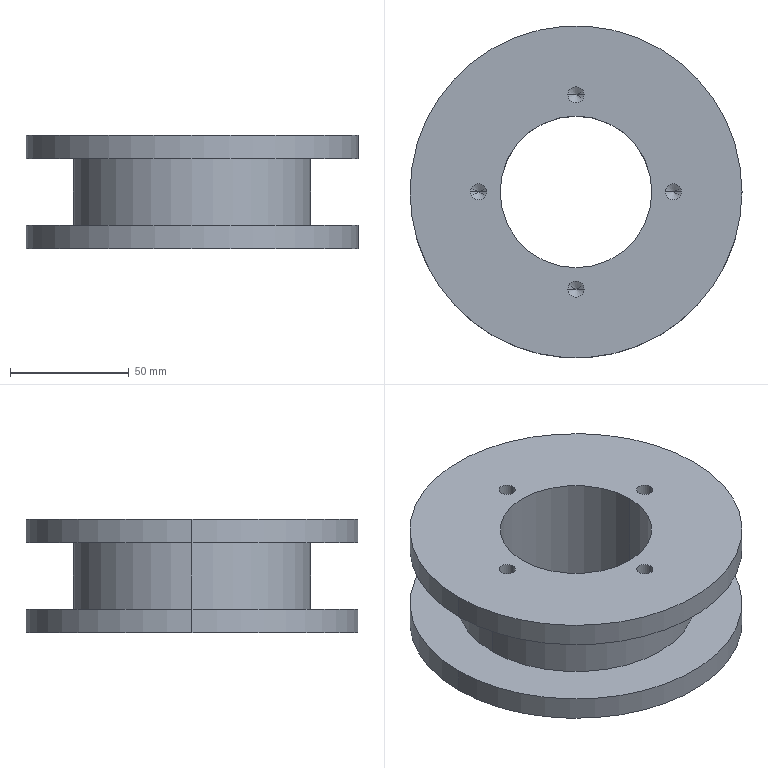Part | SolidWorks | features HoleWzd 2, Revolution 1 | 1 solid | 44 faces | box 140 x 140 x 48 mm | volume 367436 mm3 | cylinder 24 | cone 16 | plane 4 | commonest cylinder face diameters 6.8 x16 140 x4 64 x2 100 x2
STEP:
#1=CARTESIAN_POINT('',(37.6,0.,-19.75));
#2=VERTEX_POINT('',#1);
#3=CARTESIAN_POINT('',(44.4,0.,-19.75));
#4=VERTEX_POINT('',#3);
#5=CARTESIAN_POINT('',(41.,0.,-19.75));
#6=DIRECTION('',(0.,0.,1.));
#7=DIRECTION('',(1.,0.,0.));
#8=AXIS2_PLACEMENT_3D('',#5,#6,#7);
#9=CIRCLE('',#8,3.4);
#10=EDGE_CURVE('',#2,#4,#9,.T.);
#11=ORIENTED_EDGE('',*,*,#10,.F.);
#12=CARTESIAN_POINT('',(37.6,0.,0.));
#13=VERTEX_POINT('',#12);
#14=CARTESIAN_POINT('',(37.6,0.,0.));
#15=DIRECTION('',(0.,0.,1.));
#16=VECTOR('',#15,1000.);
#17=LINE('',#14,#16);
#18=EDGE_CURVE('',#2,#13,#17,.T.);
#19=ORIENTED_EDGE('',*,*,#18,.T.);
#20=CARTESIAN_POINT('',(44.4,0.,0.));
#21=VERTEX_POINT('',#20);
#22=CARTESIAN_POINT('',(41.,0.,0.));
#23=DIRECTION('',(0.,0.,1.));
#24=DIRECTION('',(1.,0.,0.));
#25=AXIS2_PLACEMENT_3D('',#22,#23,#24);
#26=CIRCLE('',#25,3.4);
#27=EDGE_CURVE('',#13,#21,#26,.T.);
#28=ORIENTED_EDGE('',*,*,#27,.T.);
#29=CARTESIAN_POINT('',(44.4,0.,0.));
#30=DIRECTION('',(0.,0.,1.));
#31=VECTOR('',#30,1000.);
#32=LINE('',#29,#31);
#33=EDGE_CURVE('',#4,#21,#32,.T.);
#34=ORIENTED_EDGE('',*,*,#33,.F.);
#35=EDGE_LOOP('',(#11,#19,#28,#34));
#36=FACE_OUTER_BOUND('',#35,.T.);
#37=CARTESIAN_POINT('',(41.,0.,0.));
#38=DIRECTION('',(0.,0.,1.));
#39=DIRECTION('',(1.,0.,0.));
#40=AXIS2_PLACEMENT_3D('',#37,#38,#39);
#41=CYLINDRICAL_SURFACE('',#40,3.4);
#42=ADVANCED_FACE('',(#36),#41,.F.);
#43=CARTESIAN_POINT('',(41.,0.,-21.793));
#44=VERTEX_POINT('',#43);
#45=CARTESIAN_POINT('',(44.4,0.,-19.75));
#46=DIRECTION('',(0.8572,0.,0.515));
#47=VECTOR('',#46,1000.);
#48=LINE('',#45,#47);
#49=EDGE_CURVE('',#44,#4,#48,.T.);
#50=ORIENTED_EDGE('',*,*,#49,.F.);
#51=CARTESIAN_POINT('',(37.6,0.,-19.75));
#52=DIRECTION('',(-0.8572,0.,0.515));
#53=VECTOR('',#52,1000.);
#54=LINE('',#51,#53);
#55=EDGE_CURVE('',#44,#2,#54,.T.);
#56=ORIENTED_EDGE('',*,*,#55,.T.);
#57=ORIENTED_EDGE('',*,*,#10,.T.);
#58=EDGE_LOOP('',(#50,#56,#57));
#59=FACE_OUTER_BOUND('',#58,.T.);
#60=CARTESIAN_POINT('',(41.,0.,-19.75));
#61=DIRECTION('',(0.,0.,1.));
#62=DIRECTION('',(1.,0.,0.));
#63=AXIS2_PLACEMENT_3D('',#60,#61,#62);
#64=CONICAL_SURFACE('',#63,3.4,1.03);
#65=ADVANCED_FACE('',(#59),#64,.F.);
#66=CARTESIAN_POINT('',(-3.4,-41.,-19.75));
#67=VERTEX_POINT('',#66);
#68=CARTESIAN_POINT('',(3.4,-41.,-19.75));
#69=VERTEX_POINT('',#68);
#70=CARTESIAN_POINT('',(0.,-41.,-19.75));
#71=DIRECTION('',(0.,0.,1.));
#72=DIRECTION('',(1.,0.,0.));
#73=AXIS2_PLACEMENT_3D('',#70,#71,#72);
#74=CIRCLE('',#73,3.4);
#75=EDGE_CURVE('',#67,#69,#74,.T.);
#76=ORIENTED_EDGE('',*,*,#75,.F.);
#77=CARTESIAN_POINT('',(-3.4,-41.,0.));
#78=VERTEX_POINT('',#77);
#79=CARTESIAN_POINT('',(-3.4,-41.,0.));
#80=DIRECTION('',(0.,0.,1.));
#81=VECTOR('',#80,1000.);
#82=LINE('',#79,#81);
#83=EDGE_CURVE('',#67,#78,#82,.T.);
#84=ORIENTED_EDGE('',*,*,#83,.T.);
#85=CARTESIAN_POINT('',(3.4,-41.,0.));
#86=VERTEX_POINT('',#85);
#87=CARTESIAN_POINT('',(0.,-41.,0.));
#88=DIRECTION('',(0.,0.,1.));
#89=DIRECTION('',(1.,0.,0.));
#90=AXIS2_PLACEMENT_3D('',#87,#88,#89);
#91=CIRCLE('',#90,3.4);
#92=EDGE_CURVE('',#78,#86,#91,.T.);
#93=ORIENTED_EDGE('',*,*,#92,.T.);
#94=CARTESIAN_POINT('',(3.4,-41.,0.));
#95=DIRECTION('',(0.,0.,1.));
#96=VECTOR('',#95,1000.);
#97=LINE('',#94,#96);
#98=EDGE_CURVE('',#69,#86,#97,.T.);
#99=ORIENTED_EDGE('',*,*,#98,.F.);
#100=EDGE_LOOP('',(#76,#84,#93,#99));
#101=FACE_OUTER_BOUND('',#100,.T.);
#102=CARTESIAN_POINT('',(0.,-41.,0.));
#103=DIRECTION('',(0.,0.,1.));
#104=DIRECTION('',(1.,0.,0.));
#105=AXIS2_PLACEMENT_3D('',#102,#103,#104);
#106=CYLINDRICAL_SURFACE('',#105,3.4);
#107=ADVANCED_FACE('',(#101),#106,.F.);
#108=CARTESIAN_POINT('',(0.,-41.,-21.793));
#109=VERTEX_POINT('',#108);
#110=CARTESIAN_POINT('',(3.4,-41.,-19.75));
#111=DIRECTION('',(0.8572,0.,0.515));
#112=VECTOR('',#111,1000.);
#113=LINE('',#110,#112);
#114=EDGE_CURVE('',#109,#69,#113,.T.);
#115=ORIENTED_EDGE('',*,*,#114,.F.);
#116=CARTESIAN_POINT('',(-3.4,-41.,-19.75));
#117=DIRECTION('',(-0.8572,0.,0.515));
#118=VECTOR('',#117,1000.);
#119=LINE('',#116,#118);
#120=EDGE_CURVE('',#109,#67,#119,.T.);
#121=ORIENTED_EDGE('',*,*,#120,.T.);
#122=ORIENTED_EDGE('',*,*,#75,.T.);
#123=EDGE_LOOP('',(#115,#121,#122));
#124=FACE_OUTER_BOUND('',#123,.T.);
#125=CARTESIAN_POINT('',(0.,-41.,-19.75));
#126=DIRECTION('',(0.,0.,1.));
#127=DIRECTION('',(1.,0.,0.));
#128=AXIS2_PLACEMENT_3D('',#125,#126,#127);
#129=CONICAL_SURFACE('',#128,3.4,1.03);
#130=ADVANCED_FACE('',(#124),#129,.F.);
#131=CARTESIAN_POINT('',(-44.4,0.,-19.75));
#132=VERTEX_POINT('',#131);
#133=CARTESIAN_POINT('',(-37.6,0.,-19.75));
#134=VERTEX_POINT('',#133);
#135=CARTESIAN_POINT('',(-41.,0.,-19.75));
#136=DIRECTION('',(0.,0.,1.));
#137=DIRECTION('',(1.,0.,0.));
#138=AXIS2_PLACEMENT_3D('',#135,#136,#137);
#139=CIRCLE('',#138,3.4);
#140=EDGE_CURVE('',#132,#134,#139,.T.);
#141=ORIENTED_EDGE('',*,*,#140,.F.);
#142=CARTESIAN_POINT('',(-44.4,0.,0.));
#143=VERTEX_POINT('',#142);
#144=CARTESIAN_POINT('',(-44.4,0.,0.));
#145=DIRECTION('',(0.,0.,1.));
#146=VECTOR('',#145,1000.);
#147=LINE('',#144,#146);
#148=EDGE_CURVE('',#132,#143,#147,.T.);
#149=ORIENTED_EDGE('',*,*,#148,.T.);
#150=CARTESIAN_POINT('',(-37.6,0.,0.));
#151=VERTEX_POINT('',#150);
#152=CARTESIAN_POINT('',(-41.,0.,0.));
#153=DIRECTION('',(0.,0.,1.));
#154=DIRECTION('',(1.,0.,0.));
#155=AXIS2_PLACEMENT_3D('',#152,#153,#154);
#156=CIRCLE('',#155,3.4);
#157=EDGE_CURVE('',#143,#151,#156,.T.);
#158=ORIENTED_EDGE('',*,*,#157,.T.);
#159=CARTESIAN_POINT('',(-37.6,0.,0.));
#160=DIRECTION('',(0.,0.,1.));
#161=VECTOR('',#160,1000.);
#162=LINE('',#159,#161);
#163=EDGE_CURVE('',#134,#151,#162,.T.);
#164=ORIENTED_EDGE('',*,*,#163,.F.);
#165=EDGE_LOOP('',(#141,#149,#158,#164));
#166=FACE_OUTER_BOUND('',#165,.T.);
#167=CARTESIAN_POINT('',(-41.,0.,0.));
#168=DIRECTION('',(0.,0.,1.));
#169=DIRECTION('',(1.,0.,0.));
#170=AXIS2_PLACEMENT_3D('',#167,#168,#169);
#171=CYLINDRICAL_SURFACE('',#170,3.4);
#172=ADVANCED_FACE('',(#166),#171,.F.);
#173=CARTESIAN_POINT('',(-41.,0.,-21.793));
#174=VERTEX_POINT('',#173);
#175=CARTESIAN_POINT('',(-37.6,0.,-19.75));
#176=DIRECTION('',(0.8572,0.,0.515));
#177=VECTOR('',#176,1000.);
#178=LINE('',#175,#177);
#179=EDGE_CURVE('',#174,#134,#178,.T.);
#180=ORIENTED_EDGE('',*,*,#179,.F.);
#181=CARTESIAN_POINT('',(-44.4,0.,-19.75));
#182=DIRECTION('',(-0.8572,0.,0.515));
#183=VECTOR('',#182,1000.);
#184=LINE('',#181,#183);
#185=EDGE_CURVE('',#174,#132,#184,.T.);
#186=ORIENTED_EDGE('',*,*,#185,.T.);
#187=ORIENTED_EDGE('',*,*,#140,.T.);
#188=EDGE_LOOP('',(#180,#186,#187));
#189=FACE_OUTER_BOUND('',#188,.T.);
#190=CARTESIAN_POINT('',(-41.,0.,-19.75));
#191=DIRECTION('',(0.,0.,1.));
#192=DIRECTION('',(1.,0.,0.));
#193=AXIS2_PLACEMENT_3D('',#190,#191,#192);
#194=CONICAL_SURFACE('',#193,3.4,1.03);
#195=ADVANCED_FACE('',(#189),#194,.F.);
#196=CARTESIAN_POINT('',(-3.4,41.,-19.75));
#197=VERTEX_POINT('',#196);
#198=CARTESIAN_POINT('',(3.4,41.,-19.75));
#199=VERTEX_POINT('',#198);
#200=CARTESIAN_POINT('',(0.,41.,-19.75));
#201=DIRECTION('',(0.,0.,1.));
#202=DIRECTION('',(1.,0.,0.));
#203=AXIS2_PLACEMENT_3D('',#200,#201,#202);
#204=CIRCLE('',#203,3.4);
#205=EDGE_CURVE('',#197,#199,#204,.T.);
#206=ORIENTED_EDGE('',*,*,#205,.F.);
#207=CARTESIAN_POINT('',(-3.4,41.,0.));
#208=VERTEX_POINT('',#207);
#209=CARTESIAN_POINT('',(-3.4,41.,0.));
#210=DIRECTION('',(0.,0.,1.));
#211=VECTOR('',#210,1000.);
#212=LINE('',#209,#211);
#213=EDGE_CURVE('',#197,#208,#212,.T.);
#214=ORIENTED_EDGE('',*,*,#213,.T.);
#215=CARTESIAN_POINT('',(3.4,41.,0.));
#216=VERTEX_POINT('',#215);
#217=CARTESIAN_POINT('',(0.,41.,0.));
#218=DIRECTION('',(0.,0.,1.));
#219=DIRECTION('',(1.,0.,0.));
#220=AXIS2_PLACEMENT_3D('',#217,#218,#219);
#221=CIRCLE('',#220,3.4);
#222=EDGE_CURVE('',#208,#216,#221,.T.);
#223=ORIENTED_EDGE('',*,*,#222,.T.);
#224=CARTESIAN_POINT('',(3.4,41.,0.));
#225=DIRECTION('',(0.,0.,1.));
#226=VECTOR('',#225,1000.);
#227=LINE('',#224,#226);
#228=EDGE_CURVE('',#199,#216,#227,.T.);
#229=ORIENTED_EDGE('',*,*,#228,.F.);
#230=EDGE_LOOP('',(#206,#214,#223,#229));
#231=FACE_OUTER_BOUND('',#230,.T.);
#232=CARTESIAN_POINT('',(0.,41.,0.));
#233=DIRECTION('',(0.,0.,1.));
#234=DIRECTION('',(1.,0.,0.));
#235=AXIS2_PLACEMENT_3D('',#232,#233,#234);
#236=CYLINDRICAL_SURFACE('',#235,3.4);
#237=ADVANCED_FACE('',(#231),#236,.F.);
#238=CARTESIAN_POINT('',(0.,41.,-21.793));
#239=VERTEX_POINT('',#238);
#240=CARTESIAN_POINT('',(3.4,41.,-19.75));
#241=DIRECTION('',(0.8572,0.,0.515));
#242=VECTOR('',#241,1000.);
#243=LINE('',#240,#242);
#244=EDGE_CURVE('',#239,#199,#243,.T.);
#245=ORIENTED_EDGE('',*,*,#244,.F.);
#246=CARTESIAN_POINT('',(-3.4,41.,-19.75));
#247=DIRECTION('',(-0.8572,0.,0.515));
#248=VECTOR('',#247,1000.);
#249=LINE('',#246,#248);
#250=EDGE_CURVE('',#239,#197,#249,.T.);
#251=ORIENTED_EDGE('',*,*,#250,.T.);
#252=ORIENTED_EDGE('',*,*,#205,.T.);
#253=EDGE_LOOP('',(#245,#251,#252));
#254=FACE_OUTER_BOUND('',#253,.T.);
#255=CARTESIAN_POINT('',(0.,41.,-19.75));
#256=DIRECTION('',(0.,0.,1.));
#257=DIRECTION('',(1.,0.,0.));
#258=AXIS2_PLACEMENT_3D('',#255,#256,#257);
#259=CONICAL_SURFACE('',#258,3.4,1.03);
#260=ADVANCED_FACE('',(#254),#259,.F.);
#261=CARTESIAN_POINT('',(3.4,41.,-28.25));
#262=VERTEX_POINT('',#261);
#263=CARTESIAN_POINT('',(-3.4,41.,-28.25));
#264=VERTEX_POINT('',#263);
#265=CARTESIAN_POINT('',(0.,41.,-28.25));
#266=DIRECTION('',(0.,0.,-1.));
#267=DIRECTION('',(-1.,0.,0.));
#268=AXIS2_PLACEMENT_3D('',#265,#266,#267);
#269=CIRCLE('',#268,3.4);
#270=EDGE_CURVE('',#262,#264,#269,.T.);
#271=ORIENTED_EDGE('',*,*,#270,.F.);
#272=CARTESIAN_POINT('',(3.4,41.,-48.));
#273=VERTEX_POINT('',#272);
#274=CARTESIAN_POINT('',(3.4,41.,-48.));
#275=DIRECTION('',(0.,0.,-1.));
#276=VECTOR('',#275,1000.);
#277=LINE('',#274,#276);
#278=EDGE_CURVE('',#262,#273,#277,.T.);
#279=ORIENTED_EDGE('',*,*,#278,.T.);
#280=CARTESIAN_POINT('',(-3.4,41.,-48.));
#281=VERTEX_POINT('',#280);
#282=CARTESIAN_POINT('',(0.,41.,-48.));
#283=DIRECTION('',(0.,0.,-1.));
#284=DIRECTION('',(-1.,0.,0.));
#285=AXIS2_PLACEMENT_3D('',#282,#283,#284);
#286=CIRCLE('',#285,3.4);
#287=EDGE_CURVE('',#273,#281,#286,.T.);
#288=ORIENTED_EDGE('',*,*,#287,.T.);
#289=CARTESIAN_POINT('',(-3.4,41.,-48.));
#290=DIRECTION('',(0.,0.,-1.));
#291=VECTOR('',#290,1000.);
#292=LINE('',#289,#291);
#293=EDGE_CURVE('',#264,#281,#292,.T.);
#294=ORIENTED_EDGE('',*,*,#293,.F.);
#295=EDGE_LOOP('',(#271,#279,#288,#294));
#296=FACE_OUTER_BOUND('',#295,.T.);
#297=CARTESIAN_POINT('',(0.,41.,-48.));
#298=DIRECTION('',(0.,0.,-1.));
#299=DIRECTION('',(-1.,0.,0.));
#300=AXIS2_PLACEMENT_3D('',#297,#298,#299);
#301=CYLINDRICAL_SURFACE('',#300,3.4);
#302=ADVANCED_FACE('',(#296),#301,.F.);
#303=CARTESIAN_POINT('',(0.,41.,-26.207));
#304=VERTEX_POINT('',#303);
#305=CARTESIAN_POINT('',(-3.4,41.,-28.25));
#306=DIRECTION('',(-0.8572,0.,-0.515));
#307=VECTOR('',#306,1000.);
#308=LINE('',#305,#307);
#309=EDGE_CURVE('',#304,#264,#308,.T.);
#310=ORIENTED_EDGE('',*,*,#309,.F.);
#311=CARTESIAN_POINT('',(3.4,41.,-28.25));
#312=DIRECTION('',(0.8572,0.,-0.515));
#313=VECTOR('',#312,1000.);
#314=LINE('',#311,#313);
#315=EDGE_CURVE('',#304,#262,#314,.T.);
#316=ORIENTED_EDGE('',*,*,#315,.T.);
#317=ORIENTED_EDGE('',*,*,#270,.T.);
#318=EDGE_LOOP('',(#310,#316,#317));
#319=FACE_OUTER_BOUND('',#318,.T.);
#320=CARTESIAN_POINT('',(0.,41.,-28.25));
#321=DIRECTION('',(0.,0.,-1.));
#322=DIRECTION('',(-1.,0.,0.));
#323=AXIS2_PLACEMENT_3D('',#320,#321,#322);
#324=CONICAL_SURFACE('',#323,3.4,1.03);
#325=ADVANCED_FACE('',(#319),#324,.F.);
#326=CARTESIAN_POINT('',(-37.6,0.,-28.25));
#327=VERTEX_POINT('',#326);
#328=CARTESIAN_POINT('',(-44.4,0.,-28.25));
#329=VERTEX_POINT('',#328);
#330=CARTESIAN_POINT('',(-41.,0.,-28.25));
#331=DIRECTION('',(0.,0.,-1.));
#332=DIRECTION('',(-1.,0.,0.));
#333=AXIS2_PLACEMENT_3D('',#330,#331,#332);
#334=CIRCLE('',#333,3.4);
#335=EDGE_CURVE('',#327,#329,#334,.T.);
#336=ORIENTED_EDGE('',*,*,#335,.F.);
#337=CARTESIAN_POINT('',(-37.6,0.,-48.));
#338=VERTEX_POINT('',#337);
#339=CARTESIAN_POINT('',(-37.6,0.,-48.));
#340=DIRECTION('',(0.,0.,-1.));
#341=VECTOR('',#340,1000.);
#342=LINE('',#339,#341);
#343=EDGE_CURVE('',#327,#338,#342,.T.);
#344=ORIENTED_EDGE('',*,*,#343,.T.);
#345=CARTESIAN_POINT('',(-44.4,0.,-48.));
#346=VERTEX_POINT('',#345);
#347=CARTESIAN_POINT('',(-41.,0.,-48.));
#348=DIRECTION('',(0.,0.,-1.));
#349=DIRECTION('',(-1.,0.,0.));
#350=AXIS2_PLACEMENT_3D('',#347,#348,#349);
#351=CIRCLE('',#350,3.4);
#352=EDGE_CURVE('',#338,#346,#351,.T.);
#353=ORIENTED_EDGE('',*,*,#352,.T.);
#354=CARTESIAN_POINT('',(-44.4,0.,-48.));
#355=DIRECTION('',(0.,0.,-1.));
#356=VECTOR('',#355,1000.);
#357=LINE('',#354,#356);
#358=EDGE_CURVE('',#329,#346,#357,.T.);
#359=ORIENTED_EDGE('',*,*,#358,.F.);
#360=EDGE_LOOP('',(#336,#344,#353,#359));
#361=FACE_OUTER_BOUND('',#360,.T.);
#362=CARTESIAN_POINT('',(-41.,0.,-48.));
#363=DIRECTION('',(0.,0.,-1.));
#364=DIRECTION('',(-1.,0.,0.));
#365=AXIS2_PLACEMENT_3D('',#362,#363,#364);
#366=CYLINDRICAL_SURFACE('',#365,3.4);
#367=ADVANCED_FACE('',(#361),#366,.F.);
#368=CARTESIAN_POINT('',(-41.,0.,-26.207));
#369=VERTEX_POINT('',#368);
#370=CARTESIAN_POINT('',(-44.4,0.,-28.25));
#371=DIRECTION('',(-0.8572,0.,-0.515));
#372=VECTOR('',#371,1000.);
#373=LINE('',#370,#372);
#374=EDGE_CURVE('',#369,#329,#373,.T.);
#375=ORIENTED_EDGE('',*,*,#374,.F.);
#376=CARTESIAN_POINT('',(-37.6,0.,-28.25));
#377=DIRECTION('',(0.8572,0.,-0.515));
#378=VECTOR('',#377,1000.);
#379=LINE('',#376,#378);
#380=EDGE_CURVE('',#369,#327,#379,.T.);
#381=ORIENTED_EDGE('',*,*,#380,.T.);
#382=ORIENTED_EDGE('',*,*,#335,.T.);
#383=EDGE_LOOP('',(#375,#381,#382));
#384=FACE_OUTER_BOUND('',#383,.T.);
#385=CARTESIAN_POINT('',(-41.,0.,-28.25));
#386=DIRECTION('',(0.,0.,-1.));
#387=DIRECTION('',(-1.,0.,0.));
#388=AXIS2_PLACEMENT_3D('',#385,#386,#387);
#389=CONICAL_SURFACE('',#388,3.4,1.03);
#390=ADVANCED_FACE('',(#384),#389,.F.);
#391=CARTESIAN_POINT('',(44.4,0.,-28.25));
#392=VERTEX_POINT('',#391);
#393=CARTESIAN_POINT('',(37.6,0.,-28.25));
#394=VERTEX_POINT('',#393);
#395=CARTESIAN_POINT('',(41.,0.,-28.25));
#396=DIRECTION('',(0.,0.,-1.));
#397=DIRECTION('',(-1.,0.,0.));
#398=AXIS2_PLACEMENT_3D('',#395,#396,#397);
#399=CIRCLE('',#398,3.4);
#400=EDGE_CURVE('',#392,#394,#399,.T.);
#401=ORIENTED_EDGE('',*,*,#400,.F.);
#402=CARTESIAN_POINT('',(44.4,0.,-48.));
#403=VERTEX_POINT('',#402);
#404=CARTESIAN_POINT('',(44.4,0.,-48.));
#405=DIRECTION('',(0.,0.,-1.));
#406=VECTOR('',#405,1000.);
#407=LINE('',#404,#406);
#408=EDGE_CURVE('',#392,#403,#407,.T.);
#409=ORIENTED_EDGE('',*,*,#408,.T.);
#410=CARTESIAN_POINT('',(37.6,0.,-48.));
#411=VERTEX_POINT('',#410);
#412=CARTESIAN_POINT('',(41.,0.,-48.));
#413=DIRECTION('',(0.,0.,-1.));
#414=DIRECTION('',(-1.,0.,0.));
#415=AXIS2_PLACEMENT_3D('',#412,#413,#414);
#416=CIRCLE('',#415,3.4);
#417=EDGE_CURVE('',#403,#411,#416,.T.);
#418=ORIENTED_EDGE('',*,*,#417,.T.);
#419=CARTESIAN_POINT('',(37.6,0.,-48.));
#420=DIRECTION('',(0.,0.,-1.));
#421=VECTOR('',#420,1000.);
#422=LINE('',#419,#421);
#423=EDGE_CURVE('',#394,#411,#422,.T.);
#424=ORIENTED_EDGE('',*,*,#423,.F.);
#425=EDGE_LOOP('',(#401,#409,#418,#424));
#426=FACE_OUTER_BOUND('',#425,.T.);
#427=CARTESIAN_POINT('',(41.,0.,-48.));
#428=DIRECTION('',(0.,0.,-1.));
#429=DIRECTION('',(-1.,0.,0.));
#430=AXIS2_PLACEMENT_3D('',#427,#428,#429);
#431=CYLINDRICAL_SURFACE('',#430,3.4);
#432=ADVANCED_FACE('',(#426),#431,.F.);
#433=CARTESIAN_POINT('',(41.,0.,-26.207));
#434=VERTEX_POINT('',#433);
#435=CARTESIAN_POINT('',(37.6,0.,-28.25));
#436=DIRECTION('',(-0.8572,0.,-0.515));
#437=VECTOR('',#436,1000.);
#438=LINE('',#435,#437);
#439=EDGE_CURVE('',#434,#394,#438,.T.);
#440=ORIENTED_EDGE('',*,*,#439,.F.);
#441=CARTESIAN_POINT('',(44.4,0.,-28.25));
#442=DIRECTION('',(0.8572,0.,-0.515));
#443=VECTOR('',#442,1000.);
#444=LINE('',#441,#443);
#445=EDGE_CURVE('',#434,#392,#444,.T.);
#446=ORIENTED_EDGE('',*,*,#445,.T.);
#447=ORIENTED_EDGE('',*,*,#400,.T.);
#448=EDGE_LOOP('',(#440,#446,#447));
#449=FACE_OUTER_BOUND('',#448,.T.);
#450=CARTESIAN_POINT('',(41.,0.,-28.25));
#451=DIRECTION('',(0.,0.,-1.));
#452=DIRECTION('',(-1.,0.,0.));
#453=AXIS2_PLACEMENT_3D('',#450,#451,#452);
#454=CONICAL_SURFACE('',#453,3.4,1.03);
#455=ADVANCED_FACE('',(#449),#454,.F.);
#456=CARTESIAN_POINT('',(3.4,-41.,-28.25));
#457=VERTEX_POINT('',#456);
#458=CARTESIAN_POINT('',(-3.4,-41.,-28.25));
#459=VERTEX_POINT('',#458);
#460=CARTESIAN_POINT('',(0.,-41.,-28.25));
#461=DIRECTION('',(0.,0.,-1.));
#462=DIRECTION('',(-1.,0.,0.));
#463=AXIS2_PLACEMENT_3D('',#460,#461,#462);
#464=CIRCLE('',#463,3.4);
#465=EDGE_CURVE('',#457,#459,#464,.T.);
#466=ORIENTED_EDGE('',*,*,#465,.F.);
#467=CARTESIAN_POINT('',(3.4,-41.,-48.));
#468=VERTEX_POINT('',#467);
#469=CARTESIAN_POINT('',(3.4,-41.,-48.));
#470=DIRECTION('',(0.,0.,-1.));
#471=VECTOR('',#470,1000.);
#472=LINE('',#469,#471);
#473=EDGE_CURVE('',#457,#468,#472,.T.);
#474=ORIENTED_EDGE('',*,*,#473,.T.);
#475=CARTESIAN_POINT('',(-3.4,-41.,-48.));
#476=VERTEX_POINT('',#475);
#477=CARTESIAN_POINT('',(0.,-41.,-48.));
#478=DIRECTION('',(0.,0.,-1.));
#479=DIRECTION('',(-1.,0.,0.));
#480=AXIS2_PLACEMENT_3D('',#477,#478,#479);
#481=CIRCLE('',#480,3.4);
#482=EDGE_CURVE('',#468,#476,#481,.T.);
#483=ORIENTED_EDGE('',*,*,#482,.T.);
#484=CARTESIAN_POINT('',(-3.4,-41.,-48.));
#485=DIRECTION('',(0.,0.,-1.));
#486=VECTOR('',#485,1000.);
#487=LINE('',#484,#486);
#488=EDGE_CURVE('',#459,#476,#487,.T.);
#489=ORIENTED_EDGE('',*,*,#488,.F.);
#490=EDGE_LOOP('',(#466,#474,#483,#489));
#491=FACE_OUTER_BOUND('',#490,.T.);
#492=CARTESIAN_POINT('',(0.,-41.,-48.));
#493=DIRECTION('',(0.,0.,-1.));
#494=DIRECTION('',(-1.,0.,0.));
#495=AXIS2_PLACEMENT_3D('',#492,#493,#494);
#496=CYLINDRICAL_SURFACE('',#495,3.4);
#497=ADVANCED_FACE('',(#491),#496,.F.);
#498=CARTESIAN_POINT('',(0.,-41.,-26.207));
#499=VERTEX_POINT('',#498);
#500=CARTESIAN_POINT('',(-3.4,-41.,-28.25));
#501=DIRECTION('',(-0.8572,0.,-0.515));
#502=VECTOR('',#501,1000.);
#503=LINE('',#500,#502);
#504=EDGE_CURVE('',#499,#459,#503,.T.);
#505=ORIENTED_EDGE('',*,*,#504,.F.);
#506=CARTESIAN_POINT('',(3.4,-41.,-28.25));
#507=DIRECTION('',(0.8572,0.,-0.515));
#508=VECTOR('',#507,1000.);
#509=LINE('',#506,#508);
#510=EDGE_CURVE('',#499,#457,#509,.T.);
#511=ORIENTED_EDGE('',*,*,#510,.T.);
#512=ORIENTED_EDGE('',*,*,#465,.T.);
#513=EDGE_LOOP('',(#505,#511,#512));
#514=FACE_OUTER_BOUND('',#513,.T.);
#515=CARTESIAN_POINT('',(0.,-41.,-28.25));
#516=DIRECTION('',(0.,0.,-1.));
#517=DIRECTION('',(-1.,0.,0.));
#518=AXIS2_PLACEMENT_3D('',#515,#516,#517);
#519=CONICAL_SURFACE('',#518,3.4,1.03);
#520=ADVANCED_FACE('',(#514),#519,.F.);
#521=CARTESIAN_POINT('',(32.,0.,0.));
#522=VERTEX_POINT('',#521);
#523=CARTESIAN_POINT('',(-32.,0.,0.));
#524=VERTEX_POINT('',#523);
#525=CARTESIAN_POINT('',(0.,0.,0.));
#526=DIRECTION('',(0.,0.,-1.));
#527=DIRECTION('',(-1.,0.,0.));
#528=AXIS2_PLACEMENT_3D('',#525,#526,#527);
#529=CIRCLE('',#528,32.);
#530=EDGE_CURVE('',#522,#524,#529,.T.);
#531=ORIENTED_EDGE('',*,*,#530,.F.);
#532=CARTESIAN_POINT('',(32.,0.,-48.));
#533=VERTEX_POINT('',#532);
#534=CARTESIAN_POINT('',(32.,0.,0.));
#535=DIRECTION('',(0.,0.,-1.));
#536=VECTOR('',#535,1000.);
#537=LINE('',#534,#536);
#538=EDGE_CURVE('',#522,#533,#537,.T.);
#539=ORIENTED_EDGE('',*,*,#538,.T.);
#540=CARTESIAN_POINT('',(-32.,0.,-48.));
#541=VERTEX_POINT('',#540);
#542=CARTESIAN_POINT('',(0.,0.,-48.));
#543=DIRECTION('',(0.,0.,-1.));
#544=DIRECTION('',(-1.,0.,0.));
#545=AXIS2_PLACEMENT_3D('',#542,#543,#544);
#546=CIRCLE('',#545,32.);
#547=EDGE_CURVE('',#533,#541,#546,.T.);
#548=ORIENTED_EDGE('',*,*,#547,.T.);
#549=CARTESIAN_POINT('',(-32.,0.,0.));
#550=DIRECTION('',(0.,0.,-1.));
#551=VECTOR('',#550,1000.);
#552=LINE('',#549,#551);
#553=EDGE_CURVE('',#524,#541,#552,.T.);
#554=ORIENTED_EDGE('',*,*,#553,.F.);
#555=EDGE_LOOP('',(#531,#539,#548,#554));
#556=FACE_OUTER_BOUND('',#555,.T.);
#557=CARTESIAN_POINT('',(0.,0.,0.));
#558=DIRECTION('',(0.,0.,-1.));
#559=DIRECTION('',(-1.,0.,0.));
#560=AXIS2_PLACEMENT_3D('',#557,#558,#559);
#561=CYLINDRICAL_SURFACE('',#560,32.);
#562=ADVANCED_FACE('',(#556),#561,.F.);
#563=CARTESIAN_POINT('',(-70.,0.,0.));
#564=VERTEX_POINT('',#563);
#565=CARTESIAN_POINT('',(70.,0.,0.));
#566=VERTEX_POINT('',#565);
#567=CARTESIAN_POINT('',(0.,0.,0.));
#568=DIRECTION('',(0.,0.,-1.));
#569=DIRECTION('',(-1.,0.,0.));
#570=AXIS2_PLACEMENT_3D('',#567,#568,#569);
#571=CIRCLE('',#570,70.);
#572=EDGE_CURVE('',#564,#566,#571,.T.);
#573=ORIENTED_EDGE('',*,*,#572,.T.);
#574=CARTESIAN_POINT('',(70.,0.,-10.));
#575=VERTEX_POINT('',#574);
#576=CARTESIAN_POINT('',(70.,0.,0.));
#577=DIRECTION('',(0.,0.,-1.));
#578=VECTOR('',#577,1000.);
#579=LINE('',#576,#578);
#580=EDGE_CURVE('',#566,#575,#579,.T.);
#581=ORIENTED_EDGE('',*,*,#580,.T.);
#582=CARTESIAN_POINT('',(-70.,0.,-10.));
#583=VERTEX_POINT('',#582);
#584=CARTESIAN_POINT('',(0.,0.,-10.));
#585=DIRECTION('',(0.,0.,-1.));
#586=DIRECTION('',(-1.,0.,0.));
#587=AXIS2_PLACEMENT_3D('',#584,#585,#586);
#588=CIRCLE('',#587,70.);
#589=EDGE_CURVE('',#583,#575,#588,.T.);
#590=ORIENTED_EDGE('',*,*,#589,.F.);
#591=CARTESIAN_POINT('',(-70.,0.,0.));
#592=DIRECTION('',(0.,0.,-1.));
#593=VECTOR('',#592,1000.);
#594=LINE('',#591,#593);
#595=EDGE_CURVE('',#564,#583,#594,.T.);
#596=ORIENTED_EDGE('',*,*,#595,.F.);
#597=EDGE_LOOP('',(#573,#581,#590,#596));
#598=FACE_OUTER_BOUND('',#597,.T.);
#599=CARTESIAN_POINT('',(0.,0.,0.));
#600=DIRECTION('',(0.,0.,-1.));
#601=DIRECTION('',(-1.,0.,0.));
#602=AXIS2_PLACEMENT_3D('',#599,#600,#601);
#603=CYLINDRICAL_SURFACE('',#602,70.);
#604=ADVANCED_FACE('',(#598),#603,.T.);
#605=CARTESIAN_POINT('',(-50.,0.,-10.));
#606=VERTEX_POINT('',#605);
#607=CARTESIAN_POINT('',(50.,0.,-10.));
#608=VERTEX_POINT('',#607);
#609=CARTESIAN_POINT('',(0.,0.,-10.));
#610=DIRECTION('',(0.,0.,-1.));
#611=DIRECTION('',(-1.,0.,0.));
#612=AXIS2_PLACEMENT_3D('',#609,#610,#611);
#613=CIRCLE('',#612,50.);
#614=EDGE_CURVE('',#606,#608,#613,.T.);
#615=ORIENTED_EDGE('',*,*,#614,.T.);
#616=CARTESIAN_POINT('',(50.,0.,-38.));
#617=VERTEX_POINT('',#616);
#618=CARTESIAN_POINT('',(50.,0.,0.));
#619=DIRECTION('',(0.,0.,-1.));
#620=VECTOR('',#619,1000.);
#621=LINE('',#618,#620);
#622=EDGE_CURVE('',#608,#617,#621,.T.);
#623=ORIENTED_EDGE('',*,*,#622,.T.);
#624=CARTESIAN_POINT('',(-50.,0.,-38.));
#625=VERTEX_POINT('',#624);
#626=CARTESIAN_POINT('',(0.,0.,-38.));
#627=DIRECTION('',(0.,0.,-1.));
#628=DIRECTION('',(-1.,0.,0.));
#629=AXIS2_PLACEMENT_3D('',#626,#627,#628);
#630=CIRCLE('',#629,50.);
#631=EDGE_CURVE('',#625,#617,#630,.T.);
#632=ORIENTED_EDGE('',*,*,#631,.F.);
#633=CARTESIAN_POINT('',(-50.,0.,0.));
#634=DIRECTION('',(0.,0.,-1.));
#635=VECTOR('',#634,1000.);
#636=LINE('',#633,#635);
#637=EDGE_CURVE('',#606,#625,#636,.T.);
#638=ORIENTED_EDGE('',*,*,#637,.F.);
#639=EDGE_LOOP('',(#615,#623,#632,#638));
#640=FACE_OUTER_BOUND('',#639,.T.);
#641=CARTESIAN_POINT('',(0.,0.,0.));
#642=DIRECTION('',(0.,0.,-1.));
#643=DIRECTION('',(-1.,0.,0.));
#644=AXIS2_PLACEMENT_3D('',#641,#642,#643);
#645=CYLINDRICAL_SURFACE('',#644,50.);
#646=ADVANCED_FACE('',(#640),#645,.T.);
#647=CARTESIAN_POINT('',(-70.,0.,-38.));
#648=VERTEX_POINT('',#647);
#649=CARTESIAN_POINT('',(70.,0.,-38.));
#650=VERTEX_POINT('',#649);
#651=CARTESIAN_POINT('',(0.,0.,-38.));
#652=DIRECTION('',(0.,0.,-1.));
#653=DIRECTION('',(-1.,0.,0.));
#654=AXIS2_PLACEMENT_3D('',#651,#652,#653);
#655=CIRCLE('',#654,70.);
#656=EDGE_CURVE('',#648,#650,#655,.T.);
#657=ORIENTED_EDGE('',*,*,#656,.T.);
#658=CARTESIAN_POINT('',(70.,0.,-48.));
#659=VERTEX_POINT('',#658);
#660=CARTESIAN_POINT('',(70.,0.,0.));
#661=DIRECTION('',(0.,0.,-1.));
#662=VECTOR('',#661,1000.);
#663=LINE('',#660,#662);
#664=EDGE_CURVE('',#650,#659,#663,.T.);
#665=ORIENTED_EDGE('',*,*,#664,.T.);
#666=CARTESIAN_POINT('',(-70.,0.,-48.));
#667=VERTEX_POINT('',#666);
#668=CARTESIAN_POINT('',(0.,0.,-48.));
#669=DIRECTION('',(0.,0.,-1.));
#670=DIRECTION('',(-1.,0.,0.));
#671=AXIS2_PLACEMENT_3D('',#668,#669,#670);
#672=CIRCLE('',#671,70.);
#673=EDGE_CURVE('',#667,#659,#672,.T.);
#674=ORIENTED_EDGE('',*,*,#673,.F.);
#675=CARTESIAN_POINT('',(-70.,0.,0.));
#676=DIRECTION('',(0.,0.,-1.));
#677=VECTOR('',#676,1000.);
#678=LINE('',#675,#677);
#679=EDGE_CURVE('',#648,#667,#678,.T.);
#680=ORIENTED_EDGE('',*,*,#679,.F.);
#681=EDGE_LOOP('',(#657,#665,#674,#680));
#682=FACE_OUTER_BOUND('',#681,.T.);
#683=CARTESIAN_POINT('',(0.,0.,0.));
#684=DIRECTION('',(0.,0.,-1.));
#685=DIRECTION('',(-1.,0.,0.));
#686=AXIS2_PLACEMENT_3D('',#683,#684,#685);
#687=CYLINDRICAL_SURFACE('',#686,70.);
#688=ADVANCED_FACE('',(#682),#687,.T.);
#689=ORIENTED_EDGE('',*,*,#664,.F.);
#690=CARTESIAN_POINT('',(0.,0.,-38.));
#691=DIRECTION('',(0.,0.,-1.));
#692=DIRECTION('',(-1.,0.,0.));
#693=AXIS2_PLACEMENT_3D('',#690,#691,#692);
#694=CIRCLE('',#693,70.);
#695=EDGE_CURVE('',#650,#648,#694,.T.);
#696=ORIENTED_EDGE('',*,*,#695,.T.);
#697=ORIENTED_EDGE('',*,*,#679,.T.);
#698=CARTESIAN_POINT('',(0.,0.,-48.));
#699=DIRECTION('',(0.,0.,-1.));
#700=DIRECTION('',(-1.,0.,0.));
#701=AXIS2_PLACEMENT_3D('',#698,#699,#700);
#702=CIRCLE('',#701,70.);
#703=EDGE_CURVE('',#659,#667,#702,.T.);
#704=ORIENTED_EDGE('',*,*,#703,.F.);
#705=EDGE_LOOP('',(#689,#696,#697,#704));
#706=FACE_OUTER_BOUND('',#705,.T.);
#707=CARTESIAN_POINT('',(0.,0.,0.));
#708=DIRECTION('',(0.,0.,-1.));
#709=DIRECTION('',(-1.,0.,0.));
#710=AXIS2_PLACEMENT_3D('',#707,#708,#709);
#711=CYLINDRICAL_SURFACE('',#710,70.);
#712=ADVANCED_FACE('',(#706),#711,.T.);
#713=ORIENTED_EDGE('',*,*,#631,.T.);
#714=CARTESIAN_POINT('',(0.,0.,-38.));
#715=DIRECTION('',(0.,0.,-1.));
#716=DIRECTION('',(-1.,0.,0.));
#717=AXIS2_PLACEMENT_3D('',#714,#715,#716);
#718=CIRCLE('',#717,50.);
#719=EDGE_CURVE('',#617,#625,#718,.T.);
#720=ORIENTED_EDGE('',*,*,#719,.T.);
#721=EDGE_LOOP('',(#713,#720));
#722=FACE_BOUND('',#721,.T.);
#723=ORIENTED_EDGE('',*,*,#656,.F.);
#724=ORIENTED_EDGE('',*,*,#695,.F.);
#725=EDGE_LOOP('',(#723,#724));
#726=FACE_OUTER_BOUND('',#725,.T.);
#727=CARTESIAN_POINT('',(-70.,0.,-38.));
#728=DIRECTION('',(0.,0.,1.));
#729=DIRECTION('',(1.,0.,0.));
#730=AXIS2_PLACEMENT_3D('',#727,#728,#729);
#731=PLANE('',#730);
#732=ADVANCED_FACE('',(#722,#726),#731,.T.);
#733=ORIENTED_EDGE('',*,*,#622,.F.);
#734=CARTESIAN_POINT('',(0.,0.,-10.));
#735=DIRECTION('',(0.,0.,-1.));
#736=DIRECTION('',(-1.,0.,0.));
#737=AXIS2_PLACEMENT_3D('',#734,#735,#736);
#738=CIRCLE('',#737,50.);
#739=EDGE_CURVE('',#608,#606,#738,.T.);
#740=ORIENTED_EDGE('',*,*,#739,.T.);
#741=ORIENTED_EDGE('',*,*,#637,.T.);
#742=ORIENTED_EDGE('',*,*,#719,.F.);
#743=EDGE_LOOP('',(#733,#740,#741,#742));
#744=FACE_OUTER_BOUND('',#743,.T.);
#745=CARTESIAN_POINT('',(0.,0.,0.));
#746=DIRECTION('',(0.,0.,-1.));
#747=DIRECTION('',(-1.,0.,0.));
#748=AXIS2_PLACEMENT_3D('',#745,#746,#747);
#749=CYLINDRICAL_SURFACE('',#748,50.);
#750=ADVANCED_FACE('',(#744),#749,.T.);
#751=ORIENTED_EDGE('',*,*,#589,.T.);
#752=CARTESIAN_POINT('',(0.,0.,-10.));
#753=DIRECTION('',(0.,0.,-1.));
#754=DIRECTION('',(-1.,0.,0.));
#755=AXIS2_PLACEMENT_3D('',#752,#753,#754);
#756=CIRCLE('',#755,70.);
#757=EDGE_CURVE('',#575,#583,#756,.T.);
#758=ORIENTED_EDGE('',*,*,#757,.T.);
#759=EDGE_LOOP('',(#751,#758));
#760=FACE_OUTER_BOUND('',#759,.T.);
#761=ORIENTED_EDGE('',*,*,#614,.F.);
#762=ORIENTED_EDGE('',*,*,#739,.F.);
#763=EDGE_LOOP('',(#761,#762));
#764=FACE_BOUND('',#763,.T.);
#765=CARTESIAN_POINT('',(-50.,0.,-10.));
#766=DIRECTION('',(0.,0.,-1.));
#767=DIRECTION('',(-1.,0.,0.));
#768=AXIS2_PLACEMENT_3D('',#765,#766,#767);
#769=PLANE('',#768);
#770=ADVANCED_FACE('',(#760,#764),#769,.T.);
#771=ORIENTED_EDGE('',*,*,#580,.F.);
#772=CARTESIAN_POINT('',(0.,0.,0.));
#773=DIRECTION('',(0.,0.,-1.));
#774=DIRECTION('',(-1.,0.,0.));
#775=AXIS2_PLACEMENT_3D('',#772,#773,#774);
#776=CIRCLE('',#775,70.);
#777=EDGE_CURVE('',#566,#564,#776,.T.);
#778=ORIENTED_EDGE('',*,*,#777,.T.);
#779=ORIENTED_EDGE('',*,*,#595,.T.);
#780=ORIENTED_EDGE('',*,*,#757,.F.);
#781=EDGE_LOOP('',(#771,#778,#779,#780));
#782=FACE_OUTER_BOUND('',#781,.T.);
#783=CARTESIAN_POINT('',(0.,0.,0.));
#784=DIRECTION('',(0.,0.,-1.));
#785=DIRECTION('',(-1.,0.,0.));
#786=AXIS2_PLACEMENT_3D('',#783,#784,#785);
#787=CYLINDRICAL_SURFACE('',#786,70.);
#788=ADVANCED_FACE('',(#782),#787,.T.);
#789=CARTESIAN_POINT('',(41.,0.,0.));
#790=DIRECTION('',(0.,0.,1.));
#791=DIRECTION('',(1.,0.,0.));
#792=AXIS2_PLACEMENT_3D('',#789,#790,#791);
#793=CIRCLE('',#792,3.4);
#794=EDGE_CURVE('',#21,#13,#793,.T.);
#795=ORIENTED_EDGE('',*,*,#794,.F.);
#796=ORIENTED_EDGE('',*,*,#27,.F.);
#797=EDGE_LOOP('',(#795,#796));
#798=FACE_BOUND('',#797,.T.);
#799=CARTESIAN_POINT('',(0.,-41.,0.));
#800=DIRECTION('',(0.,0.,1.));
#801=DIRECTION('',(1.,0.,0.));
#802=AXIS2_PLACEMENT_3D('',#799,#800,#801);
#803=CIRCLE('',#802,3.4);
#804=EDGE_CURVE('',#86,#78,#803,.T.);
#805=ORIENTED_EDGE('',*,*,#804,.F.);
#806=ORIENTED_EDGE('',*,*,#92,.F.);
#807=EDGE_LOOP('',(#805,#806));
#808=FACE_BOUND('',#807,.T.);
#809=CARTESIAN_POINT('',(-41.,0.,0.));
#810=DIRECTION('',(0.,0.,1.));
#811=DIRECTION('',(1.,0.,0.));
#812=AXIS2_PLACEMENT_3D('',#809,#810,#811);
#813=CIRCLE('',#812,3.4);
#814=EDGE_CURVE('',#151,#143,#813,.T.);
#815=ORIENTED_EDGE('',*,*,#814,.F.);
#816=ORIENTED_EDGE('',*,*,#157,.F.);
#817=EDGE_LOOP('',(#815,#816));
#818=FACE_BOUND('',#817,.T.);
#819=CARTESIAN_POINT('',(0.,41.,0.));
#820=DIRECTION('',(0.,0.,1.));
#821=DIRECTION('',(1.,0.,0.));
#822=AXIS2_PLACEMENT_3D('',#819,#820,#821);
#823=CIRCLE('',#822,3.4);
#824=EDGE_CURVE('',#216,#208,#823,.T.);
#825=ORIENTED_EDGE('',*,*,#824,.F.);
#826=ORIENTED_EDGE('',*,*,#222,.F.);
#827=EDGE_LOOP('',(#825,#826));
#828=FACE_BOUND('',#827,.T.);
#829=CARTESIAN_POINT('',(0.,0.,0.));
#830=DIRECTION('',(0.,0.,-1.));
#831=DIRECTION('',(-1.,0.,0.));
#832=AXIS2_PLACEMENT_3D('',#829,#830,#831);
#833=CIRCLE('',#832,32.);
#834=EDGE_CURVE('',#524,#522,#833,.T.);
#835=ORIENTED_EDGE('',*,*,#834,.T.);
#836=ORIENTED_EDGE('',*,*,#530,.T.);
#837=EDGE_LOOP('',(#835,#836));
#838=FACE_BOUND('',#837,.T.);
#839=ORIENTED_EDGE('',*,*,#572,.F.);
#840=ORIENTED_EDGE('',*,*,#777,.F.);
#841=EDGE_LOOP('',(#839,#840));
#842=FACE_OUTER_BOUND('',#841,.T.);
#843=CARTESIAN_POINT('',(-70.,0.,0.));
#844=DIRECTION('',(0.,0.,1.));
#845=DIRECTION('',(1.,0.,0.));
#846=AXIS2_PLACEMENT_3D('',#843,#844,#845);
#847=PLANE('',#846);
#848=ADVANCED_FACE('',(#798,#808,#818,#828,#838,#842),#847,.T.);
#849=ORIENTED_EDGE('',*,*,#538,.F.);
#850=ORIENTED_EDGE('',*,*,#834,.F.);
#851=ORIENTED_EDGE('',*,*,#553,.T.);
#852=CARTESIAN_POINT('',(0.,0.,-48.));
#853=DIRECTION('',(0.,0.,-1.));
#854=DIRECTION('',(-1.,0.,0.));
#855=AXIS2_PLACEMENT_3D('',#852,#853,#854);
#856=CIRCLE('',#855,32.);
#857=EDGE_CURVE('',#541,#533,#856,.T.);
#858=ORIENTED_EDGE('',*,*,#857,.T.);
#859=EDGE_LOOP('',(#849,#850,#851,#858));
#860=FACE_OUTER_BOUND('',#859,.T.);
#861=CARTESIAN_POINT('',(0.,0.,0.));
#862=DIRECTION('',(0.,0.,-1.));
#863=DIRECTION('',(-1.,0.,0.));
#864=AXIS2_PLACEMENT_3D('',#861,#862,#863);
#865=CYLINDRICAL_SURFACE('',#864,32.);
#866=ADVANCED_FACE('',(#860),#865,.F.);
#867=CARTESIAN_POINT('',(0.,41.,-48.));
#868=DIRECTION('',(0.,0.,-1.));
#869=DIRECTION('',(-1.,0.,0.));
#870=AXIS2_PLACEMENT_3D('',#867,#868,#869);
#871=CIRCLE('',#870,3.4);
#872=EDGE_CURVE('',#281,#273,#871,.T.);
#873=ORIENTED_EDGE('',*,*,#872,.F.);
#874=ORIENTED_EDGE('',*,*,#287,.F.);
#875=EDGE_LOOP('',(#873,#874));
#876=FACE_BOUND('',#875,.T.);
#877=CARTESIAN_POINT('',(-41.,0.,-48.));
#878=DIRECTION('',(0.,0.,-1.));
#879=DIRECTION('',(-1.,0.,0.));
#880=AXIS2_PLACEMENT_3D('',#877,#878,#879);
#881=CIRCLE('',#880,3.4);
#882=EDGE_CURVE('',#346,#338,#881,.T.);
#883=ORIENTED_EDGE('',*,*,#882,.F.);
#884=ORIENTED_EDGE('',*,*,#352,.F.);
#885=EDGE_LOOP('',(#883,#884));
#886=FACE_BOUND('',#885,.T.);
#887=CARTESIAN_POINT('',(41.,0.,-48.));
#888=DIRECTION('',(0.,0.,-1.));
#889=DIRECTION('',(-1.,0.,0.));
#890=AXIS2_PLACEMENT_3D('',#887,#888,#889);
#891=CIRCLE('',#890,3.4);
#892=EDGE_CURVE('',#411,#403,#891,.T.);
#893=ORIENTED_EDGE('',*,*,#892,.F.);
#894=ORIENTED_EDGE('',*,*,#417,.F.);
#895=EDGE_LOOP('',(#893,#894));
#896=FACE_BOUND('',#895,.T.);
#897=CARTESIAN_POINT('',(0.,-41.,-48.));
#898=DIRECTION('',(0.,0.,-1.));
#899=DIRECTION('',(-1.,0.,0.));
#900=AXIS2_PLACEMENT_3D('',#897,#898,#899);
#901=CIRCLE('',#900,3.4);
#902=EDGE_CURVE('',#476,#468,#901,.T.);
#903=ORIENTED_EDGE('',*,*,#902,.F.);
#904=ORIENTED_EDGE('',*,*,#482,.F.);
#905=EDGE_LOOP('',(#903,#904));
#906=FACE_BOUND('',#905,.T.);
#907=ORIENTED_EDGE('',*,*,#673,.T.);
#908=ORIENTED_EDGE('',*,*,#703,.T.);
#909=EDGE_LOOP('',(#907,#908));
#910=FACE_OUTER_BOUND('',#909,.T.);
#911=ORIENTED_EDGE('',*,*,#857,.F.);
#912=ORIENTED_EDGE('',*,*,#547,.F.);
#913=EDGE_LOOP('',(#911,#912));
#914=FACE_BOUND('',#913,.T.);
#915=CARTESIAN_POINT('',(-32.,0.,-48.));
#916=DIRECTION('',(0.,0.,-1.));
#917=DIRECTION('',(-1.,0.,0.));
#918=AXIS2_PLACEMENT_3D('',#915,#916,#917);
#919=PLANE('',#918);
#920=ADVANCED_FACE('',(#876,#886,#896,#906,#910,#914),#919,.T.);
#921=ORIENTED_EDGE('',*,*,#510,.F.);
#922=ORIENTED_EDGE('',*,*,#504,.T.);
#923=CARTESIAN_POINT('',(0.,-41.,-28.25));
#924=DIRECTION('',(0.,0.,-1.));
#925=DIRECTION('',(-1.,0.,0.));
#926=AXIS2_PLACEMENT_3D('',#923,#924,#925);
#927=CIRCLE('',#926,3.4);
#928=EDGE_CURVE('',#459,#457,#927,.T.);
#929=ORIENTED_EDGE('',*,*,#928,.T.);
#930=EDGE_LOOP('',(#921,#922,#929));
#931=FACE_OUTER_BOUND('',#930,.T.);
#932=CARTESIAN_POINT('',(0.,-41.,-28.25));
#933=DIRECTION('',(0.,0.,-1.));
#934=DIRECTION('',(-1.,0.,0.));
#935=AXIS2_PLACEMENT_3D('',#932,#933,#934);
#936=CONICAL_SURFACE('',#935,3.4,1.03);
#937=ADVANCED_FACE('',(#931),#936,.F.);
#938=ORIENTED_EDGE('',*,*,#473,.F.);
#939=ORIENTED_EDGE('',*,*,#928,.F.);
#940=ORIENTED_EDGE('',*,*,#488,.T.);
#941=ORIENTED_EDGE('',*,*,#902,.T.);
#942=EDGE_LOOP('',(#938,#939,#940,#941));
#943=FACE_OUTER_BOUND('',#942,.T.);
#944=CARTESIAN_POINT('',(0.,-41.,-48.));
#945=DIRECTION('',(0.,0.,-1.));
#946=DIRECTION('',(-1.,0.,0.));
#947=AXIS2_PLACEMENT_3D('',#944,#945,#946);
#948=CYLINDRICAL_SURFACE('',#947,3.4);
#949=ADVANCED_FACE('',(#943),#948,.F.);
#950=ORIENTED_EDGE('',*,*,#445,.F.);
#951=ORIENTED_EDGE('',*,*,#439,.T.);
#952=CARTESIAN_POINT('',(41.,0.,-28.25));
#953=DIRECTION('',(0.,0.,-1.));
#954=DIRECTION('',(-1.,0.,0.));
#955=AXIS2_PLACEMENT_3D('',#952,#953,#954);
#956=CIRCLE('',#955,3.4);
#957=EDGE_CURVE('',#394,#392,#956,.T.);
#958=ORIENTED_EDGE('',*,*,#957,.T.);
#959=EDGE_LOOP('',(#950,#951,#958));
#960=FACE_OUTER_BOUND('',#959,.T.);
#961=CARTESIAN_POINT('',(41.,0.,-28.25));
#962=DIRECTION('',(0.,0.,-1.));
#963=DIRECTION('',(-1.,0.,0.));
#964=AXIS2_PLACEMENT_3D('',#961,#962,#963);
#965=CONICAL_SURFACE('',#964,3.4,1.03);
#966=ADVANCED_FACE('',(#960),#965,.F.);
#967=ORIENTED_EDGE('',*,*,#408,.F.);
#968=ORIENTED_EDGE('',*,*,#957,.F.);
#969=ORIENTED_EDGE('',*,*,#423,.T.);
#970=ORIENTED_EDGE('',*,*,#892,.T.);
#971=EDGE_LOOP('',(#967,#968,#969,#970));
#972=FACE_OUTER_BOUND('',#971,.T.);
#973=CARTESIAN_POINT('',(41.,0.,-48.));
#974=DIRECTION('',(0.,0.,-1.));
#975=DIRECTION('',(-1.,0.,0.));
#976=AXIS2_PLACEMENT_3D('',#973,#974,#975);
#977=CYLINDRICAL_SURFACE('',#976,3.4);
#978=ADVANCED_FACE('',(#972),#977,.F.);
#979=ORIENTED_EDGE('',*,*,#380,.F.);
#980=ORIENTED_EDGE('',*,*,#374,.T.);
#981=CARTESIAN_POINT('',(-41.,0.,-28.25));
#982=DIRECTION('',(0.,0.,-1.));
#983=DIRECTION('',(-1.,0.,0.));
#984=AXIS2_PLACEMENT_3D('',#981,#982,#983);
#985=CIRCLE('',#984,3.4);
#986=EDGE_CURVE('',#329,#327,#985,.T.);
#987=ORIENTED_EDGE('',*,*,#986,.T.);
#988=EDGE_LOOP('',(#979,#980,#987));
#989=FACE_OUTER_BOUND('',#988,.T.);
#990=CARTESIAN_POINT('',(-41.,0.,-28.25));
#991=DIRECTION('',(0.,0.,-1.));
#992=DIRECTION('',(-1.,0.,0.));
#993=AXIS2_PLACEMENT_3D('',#990,#991,#992);
#994=CONICAL_SURFACE('',#993,3.4,1.03);
#995=ADVANCED_FACE('',(#989),#994,.F.);
#996=ORIENTED_EDGE('',*,*,#343,.F.);
#997=ORIENTED_EDGE('',*,*,#986,.F.);
#998=ORIENTED_EDGE('',*,*,#358,.T.);
#999=ORIENTED_EDGE('',*,*,#882,.T.);
#1000=EDGE_LOOP('',(#996,#997,#998,#999));
#1001=FACE_OUTER_BOUND('',#1000,.T.);
#1002=CARTESIAN_POINT('',(-41.,0.,-48.));
#1003=DIRECTION('',(0.,0.,-1.));
#1004=DIRECTION('',(-1.,0.,0.));
#1005=AXIS2_PLACEMENT_3D('',#1002,#1003,#1004);
#1006=CYLINDRICAL_SURFACE('',#1005,3.4);
#1007=ADVANCED_FACE('',(#1001),#1006,.F.);
#1008=ORIENTED_EDGE('',*,*,#315,.F.);
#1009=ORIENTED_EDGE('',*,*,#309,.T.);
#1010=CARTESIAN_POINT('',(0.,41.,-28.25));
#1011=DIRECTION('',(0.,0.,-1.));
#1012=DIRECTION('',(-1.,0.,0.));
#1013=AXIS2_PLACEMENT_3D('',#1010,#1011,#1012);
#1014=CIRCLE('',#1013,3.4);
#1015=EDGE_CURVE('',#264,#262,#1014,.T.);
#1016=ORIENTED_EDGE('',*,*,#1015,.T.);
#1017=EDGE_LOOP('',(#1008,#1009,#1016));
#1018=FACE_OUTER_BOUND('',#1017,.T.);
#1019=CARTESIAN_POINT('',(0.,41.,-28.25));
#1020=DIRECTION('',(0.,0.,-1.));
#1021=DIRECTION('',(-1.,0.,0.));
#1022=AXIS2_PLACEMENT_3D('',#1019,#1020,#1021);
#1023=CONICAL_SURFACE('',#1022,3.4,1.03);
#1024=ADVANCED_FACE('',(#1018),#1023,.F.);
#1025=ORIENTED_EDGE('',*,*,#278,.F.);
#1026=ORIENTED_EDGE('',*,*,#1015,.F.);
#1027=ORIENTED_EDGE('',*,*,#293,.T.);
#1028=ORIENTED_EDGE('',*,*,#872,.T.);
#1029=EDGE_LOOP('',(#1025,#1026,#1027,#1028));
#1030=FACE_OUTER_BOUND('',#1029,.T.);
#1031=CARTESIAN_POINT('',(0.,41.,-48.));
#1032=DIRECTION('',(0.,0.,-1.));
#1033=DIRECTION('',(-1.,0.,0.));
#1034=AXIS2_PLACEMENT_3D('',#1031,#1032,#1033);
#1035=CYLINDRICAL_SURFACE('',#1034,3.4);
#1036=ADVANCED_FACE('',(#1030),#1035,.F.);
#1037=ORIENTED_EDGE('',*,*,#250,.F.);
#1038=ORIENTED_EDGE('',*,*,#244,.T.);
#1039=CARTESIAN_POINT('',(0.,41.,-19.75));
#1040=DIRECTION('',(0.,0.,1.));
#1041=DIRECTION('',(1.,0.,0.));
#1042=AXIS2_PLACEMENT_3D('',#1039,#1040,#1041);
#1043=CIRCLE('',#1042,3.4);
#1044=EDGE_CURVE('',#199,#197,#1043,.T.);
#1045=ORIENTED_EDGE('',*,*,#1044,.T.);
#1046=EDGE_LOOP('',(#1037,#1038,#1045));
#1047=FACE_OUTER_BOUND('',#1046,.T.);
#1048=CARTESIAN_POINT('',(0.,41.,-19.75));
#1049=DIRECTION('',(0.,0.,1.));
#1050=DIRECTION('',(1.,0.,0.));
#1051=AXIS2_PLACEMENT_3D('',#1048,#1049,#1050);
#1052=CONICAL_SURFACE('',#1051,3.4,1.03);
#1053=ADVANCED_FACE('',(#1047),#1052,.F.);
#1054=ORIENTED_EDGE('',*,*,#213,.F.);
#1055=ORIENTED_EDGE('',*,*,#1044,.F.);
#1056=ORIENTED_EDGE('',*,*,#228,.T.);
#1057=ORIENTED_EDGE('',*,*,#824,.T.);
#1058=EDGE_LOOP('',(#1054,#1055,#1056,#1057));
#1059=FACE_OUTER_BOUND('',#1058,.T.);
#1060=CARTESIAN_POINT('',(0.,41.,0.));
#1061=DIRECTION('',(0.,0.,1.));
#1062=DIRECTION('',(1.,0.,0.));
#1063=AXIS2_PLACEMENT_3D('',#1060,#1061,#1062);
#1064=CYLINDRICAL_SURFACE('',#1063,3.4);
#1065=ADVANCED_FACE('',(#1059),#1064,.F.);
#1066=ORIENTED_EDGE('',*,*,#185,.F.);
#1067=ORIENTED_EDGE('',*,*,#179,.T.);
#1068=CARTESIAN_POINT('',(-41.,0.,-19.75));
#1069=DIRECTION('',(0.,0.,1.));
#1070=DIRECTION('',(1.,0.,0.));
#1071=AXIS2_PLACEMENT_3D('',#1068,#1069,#1070);
#1072=CIRCLE('',#1071,3.4);
#1073=EDGE_CURVE('',#134,#132,#1072,.T.);
#1074=ORIENTED_EDGE('',*,*,#1073,.T.);
#1075=EDGE_LOOP('',(#1066,#1067,#1074));
#1076=FACE_OUTER_BOUND('',#1075,.T.);
#1077=CARTESIAN_POINT('',(-41.,0.,-19.75));
#1078=DIRECTION('',(0.,0.,1.));
#1079=DIRECTION('',(1.,0.,0.));
#1080=AXIS2_PLACEMENT_3D('',#1077,#1078,#1079);
#1081=CONICAL_SURFACE('',#1080,3.4,1.03);
#1082=ADVANCED_FACE('',(#1076),#1081,.F.);
#1083=ORIENTED_EDGE('',*,*,#148,.F.);
#1084=ORIENTED_EDGE('',*,*,#1073,.F.);
#1085=ORIENTED_EDGE('',*,*,#163,.T.);
#1086=ORIENTED_EDGE('',*,*,#814,.T.);
#1087=EDGE_LOOP('',(#1083,#1084,#1085,#1086));
#1088=FACE_OUTER_BOUND('',#1087,.T.);
#1089=CARTESIAN_POINT('',(-41.,0.,0.));
#1090=DIRECTION('',(0.,0.,1.));
#1091=DIRECTION('',(1.,0.,0.));
#1092=AXIS2_PLACEMENT_3D('',#1089,#1090,#1091);
#1093=CYLINDRICAL_SURFACE('',#1092,3.4);
#1094=ADVANCED_FACE('',(#1088),#1093,.F.);
#1095=ORIENTED_EDGE('',*,*,#120,.F.);
#1096=ORIENTED_EDGE('',*,*,#114,.T.);
#1097=CARTESIAN_POINT('',(0.,-41.,-19.75));
#1098=DIRECTION('',(0.,0.,1.));
#1099=DIRECTION('',(1.,0.,0.));
#1100=AXIS2_PLACEMENT_3D('',#1097,#1098,#1099);
#1101=CIRCLE('',#1100,3.4);
#1102=EDGE_CURVE('',#69,#67,#1101,.T.);
#1103=ORIENTED_EDGE('',*,*,#1102,.T.);
#1104=EDGE_LOOP('',(#1095,#1096,#1103));
#1105=FACE_OUTER_BOUND('',#1104,.T.);
#1106=CARTESIAN_POINT('',(0.,-41.,-19.75));
#1107=DIRECTION('',(0.,0.,1.));
#1108=DIRECTION('',(1.,0.,0.));
#1109=AXIS2_PLACEMENT_3D('',#1106,#1107,#1108);
#1110=CONICAL_SURFACE('',#1109,3.4,1.03);
#1111=ADVANCED_FACE('',(#1105),#1110,.F.);
#1112=ORIENTED_EDGE('',*,*,#83,.F.);
#1113=ORIENTED_EDGE('',*,*,#1102,.F.);
#1114=ORIENTED_EDGE('',*,*,#98,.T.);
#1115=ORIENTED_EDGE('',*,*,#804,.T.);
#1116=EDGE_LOOP('',(#1112,#1113,#1114,#1115));
#1117=FACE_OUTER_BOUND('',#1116,.T.);
#1118=CARTESIAN_POINT('',(0.,-41.,0.));
#1119=DIRECTION('',(0.,0.,1.));
#1120=DIRECTION('',(1.,0.,0.));
#1121=AXIS2_PLACEMENT_3D('',#1118,#1119,#1120);
#1122=CYLINDRICAL_SURFACE('',#1121,3.4);
#1123=ADVANCED_FACE('',(#1117),#1122,.F.);
#1124=ORIENTED_EDGE('',*,*,#55,.F.);
#1125=ORIENTED_EDGE('',*,*,#49,.T.);
#1126=CARTESIAN_POINT('',(41.,0.,-19.75));
#1127=DIRECTION('',(0.,0.,1.));
#1128=DIRECTION('',(1.,0.,0.));
#1129=AXIS2_PLACEMENT_3D('',#1126,#1127,#1128);
#1130=CIRCLE('',#1129,3.4);
#1131=EDGE_CURVE('',#4,#2,#1130,.T.);
#1132=ORIENTED_EDGE('',*,*,#1131,.T.);
#1133=EDGE_LOOP('',(#1124,#1125,#1132));
#1134=FACE_OUTER_BOUND('',#1133,.T.);
#1135=CARTESIAN_POINT('',(41.,0.,-19.75));
#1136=DIRECTION('',(0.,0.,1.));
#1137=DIRECTION('',(1.,0.,0.));
#1138=AXIS2_PLACEMENT_3D('',#1135,#1136,#1137);
#1139=CONICAL_SURFACE('',#1138,3.4,1.03);
#1140=ADVANCED_FACE('',(#1134),#1139,.F.);
#1141=ORIENTED_EDGE('',*,*,#18,.F.);
#1142=ORIENTED_EDGE('',*,*,#1131,.F.);
#1143=ORIENTED_EDGE('',*,*,#33,.T.);
#1144=ORIENTED_EDGE('',*,*,#794,.T.);
#1145=EDGE_LOOP('',(#1141,#1142,#1143,#1144));
#1146=FACE_OUTER_BOUND('',#1145,.T.);
#1147=CARTESIAN_POINT('',(41.,0.,0.));
#1148=DIRECTION('',(0.,0.,1.));
#1149=DIRECTION('',(1.,0.,0.));
#1150=AXIS2_PLACEMENT_3D('',#1147,#1148,#1149);
#1151=CYLINDRICAL_SURFACE('',#1150,3.4);
#1152=ADVANCED_FACE('',(#1146),#1151,.F.);
#1153=CLOSED_SHELL('',(#42,#65,#107,#130,#172,#195,#237,#260,#302,#325,#367,#390,#432,#455,#497,#520,#562,#604,#646,#688,#712,#732,#750,#770,#788,#848,#866,#920,#937,#949,#966,#978,#995,#1007,#1024,#1036,#1053,#1065,#1082,#1094,#1111,#1123,#1140,#1152));
#1154=MANIFOLD_SOLID_BREP('',#1153);
#1155=CARTESIAN_POINT('',(0.,0.,0.));
#1156=DIRECTION('',(0.,0.,1.));
#1157=DIRECTION('',(1.,0.,0.));
#1158=AXIS2_PLACEMENT_3D('',#1155,#1156,#1157);
#1159=(LENGTH_UNIT()NAMED_UNIT(*)SI_UNIT(.MILLI.,.METRE.));
#1160=UNCERTAINTY_MEASURE_WITH_UNIT(LENGTH_MEASURE(0.00001),#1159,'','');
#1161=(NAMED_UNIT(*)PLANE_ANGLE_UNIT()SI_UNIT($,.RADIAN.));
#1162=(NAMED_UNIT(*)SI_UNIT($,.STERADIAN.)SOLID_ANGLE_UNIT());
#1163=(GEOMETRIC_REPRESENTATION_CONTEXT(3)GLOBAL_UNCERTAINTY_ASSIGNED_CONTEXT((#1160))GLOBAL_UNIT_ASSIGNED_CONTEXT((#1159,#1161,#1162))REPRESENTATION_CONTEXT('',''));
#1164=ADVANCED_BREP_SHAPE_REPRESENTATION('',(#1154,#1158),#1163);